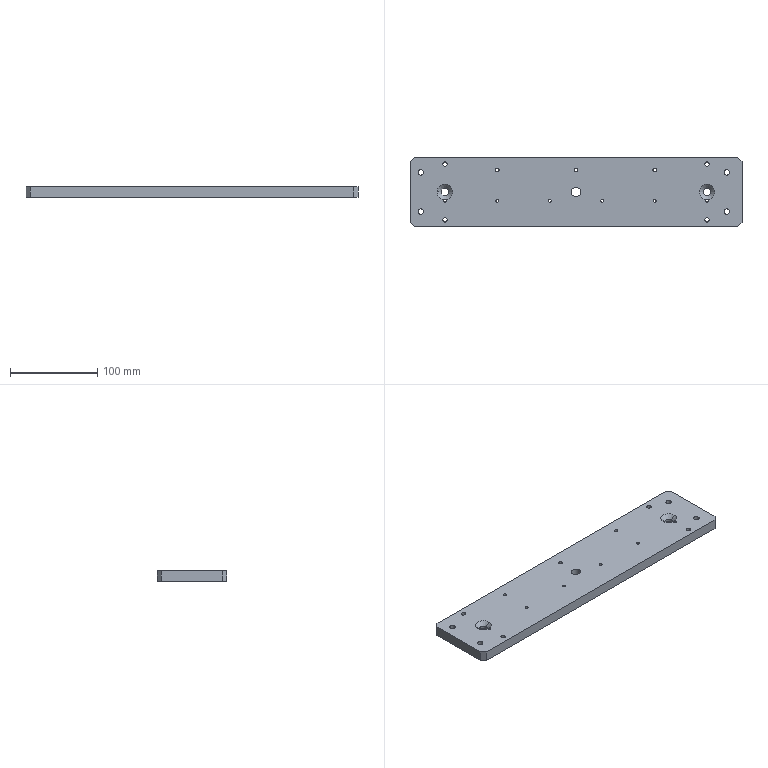Part | STEP file | Width adjustment base | 1 solid | 58 faces | box 380 x 80 x 12 mm | volume 356572 mm3 | cylinder 40 | plane 10 | cone 8 | commonest cylinder face diameters 3.3 x12 5 x8 6.2 x8 4.2 x6 9 x4 10.8 x2